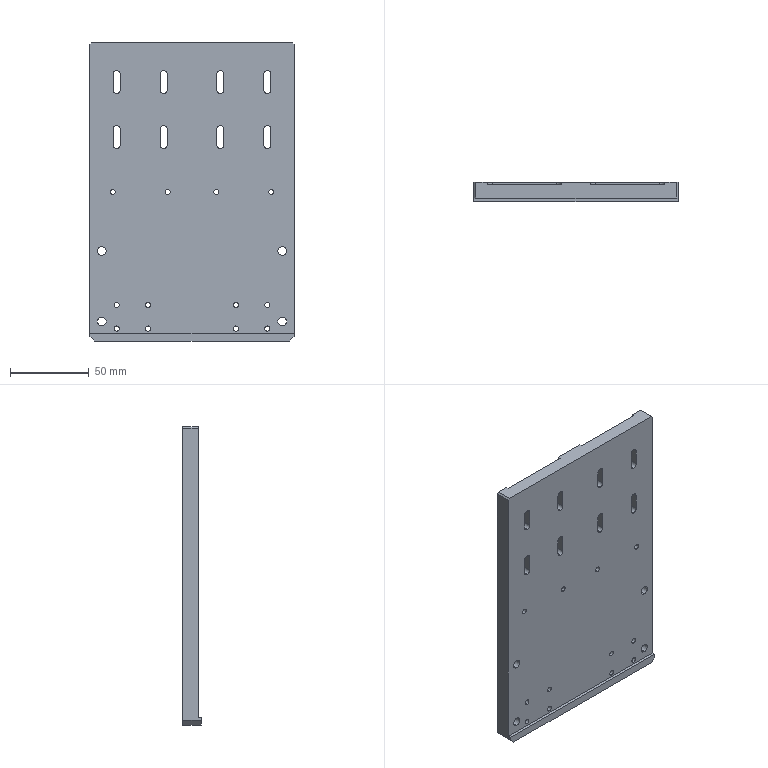Part | NX | features BREP 1 | 1 solid | 108 faces | box 130 x 12 x 190 mm | volume 228290 mm3 | cylinder 68 | plane 40 | commonest cylinder face diameters 3.3 x24 4.5 x24 5.5 x8 10 x8 6 x4